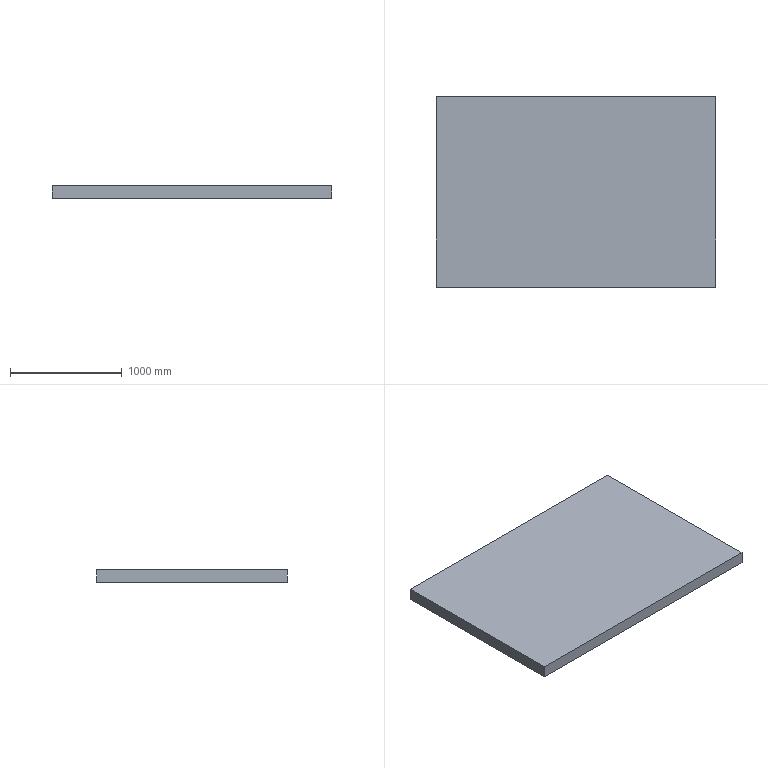Part | SolidWorks | features BaseBody 1 | 1 solid | 6 faces | box 2500 x 1700 x 110 mm | volume 467500000 mm3 | plane 6
STEP:
#1=CARTESIAN_POINT('',(1250.,-850.,0.));
#2=VERTEX_POINT('',#1);
#3=CARTESIAN_POINT('',(1250.,850.,0.));
#4=VERTEX_POINT('',#3);
#5=CARTESIAN_POINT('',(1250.,850.,0.));
#6=DIRECTION('',(0.,1.,0.));
#7=VECTOR('',#6,1000.);
#8=LINE('',#5,#7);
#9=EDGE_CURVE('',#2,#4,#8,.T.);
#10=ORIENTED_EDGE('',*,*,#9,.F.);
#11=CARTESIAN_POINT('',(-1250.,-850.,0.));
#12=VERTEX_POINT('',#11);
#13=CARTESIAN_POINT('',(-1250.,-850.,0.));
#14=DIRECTION('',(1.,0.,0.));
#15=VECTOR('',#14,1000.);
#16=LINE('',#13,#15);
#17=EDGE_CURVE('',#12,#2,#16,.T.);
#18=ORIENTED_EDGE('',*,*,#17,.F.);
#19=CARTESIAN_POINT('',(-1250.,850.,0.));
#20=VERTEX_POINT('',#19);
#21=CARTESIAN_POINT('',(-1250.,850.,0.));
#22=DIRECTION('',(0.,-1.,0.));
#23=VECTOR('',#22,1000.);
#24=LINE('',#21,#23);
#25=EDGE_CURVE('',#20,#12,#24,.T.);
#26=ORIENTED_EDGE('',*,*,#25,.F.);
#27=CARTESIAN_POINT('',(-1250.,850.,0.));
#28=DIRECTION('',(-1.,0.,0.));
#29=VECTOR('',#28,1000.);
#30=LINE('',#27,#29);
#31=EDGE_CURVE('',#4,#20,#30,.T.);
#32=ORIENTED_EDGE('',*,*,#31,.F.);
#33=EDGE_LOOP('',(#10,#18,#26,#32));
#34=FACE_OUTER_BOUND('',#33,.T.);
#35=CARTESIAN_POINT('',(0.,0.,0.));
#36=DIRECTION('',(0.,0.,1.));
#37=DIRECTION('',(1.,0.,0.));
#38=AXIS2_PLACEMENT_3D('',#35,#36,#37);
#39=PLANE('',#38);
#40=ADVANCED_FACE('',(#34),#39,.F.);
#41=CARTESIAN_POINT('',(1250.,-850.,110.));
#42=VERTEX_POINT('',#41);
#43=CARTESIAN_POINT('',(1250.,850.,110.));
#44=VERTEX_POINT('',#43);
#45=CARTESIAN_POINT('',(1250.,850.,110.));
#46=DIRECTION('',(0.,1.,0.));
#47=VECTOR('',#46,1000.);
#48=LINE('',#45,#47);
#49=EDGE_CURVE('',#42,#44,#48,.T.);
#50=ORIENTED_EDGE('',*,*,#49,.T.);
#51=CARTESIAN_POINT('',(-1250.,850.,110.));
#52=VERTEX_POINT('',#51);
#53=CARTESIAN_POINT('',(-1250.,850.,110.));
#54=DIRECTION('',(-1.,0.,0.));
#55=VECTOR('',#54,1000.);
#56=LINE('',#53,#55);
#57=EDGE_CURVE('',#44,#52,#56,.T.);
#58=ORIENTED_EDGE('',*,*,#57,.T.);
#59=CARTESIAN_POINT('',(-1250.,-850.,110.));
#60=VERTEX_POINT('',#59);
#61=CARTESIAN_POINT('',(-1250.,850.,110.));
#62=DIRECTION('',(0.,-1.,0.));
#63=VECTOR('',#62,1000.);
#64=LINE('',#61,#63);
#65=EDGE_CURVE('',#52,#60,#64,.T.);
#66=ORIENTED_EDGE('',*,*,#65,.T.);
#67=CARTESIAN_POINT('',(-1250.,-850.,110.));
#68=DIRECTION('',(1.,0.,0.));
#69=VECTOR('',#68,1000.);
#70=LINE('',#67,#69);
#71=EDGE_CURVE('',#60,#42,#70,.T.);
#72=ORIENTED_EDGE('',*,*,#71,.T.);
#73=EDGE_LOOP('',(#50,#58,#66,#72));
#74=FACE_OUTER_BOUND('',#73,.T.);
#75=CARTESIAN_POINT('',(0.,0.,110.));
#76=DIRECTION('',(0.,0.,1.));
#77=DIRECTION('',(1.,0.,0.));
#78=AXIS2_PLACEMENT_3D('',#75,#76,#77);
#79=PLANE('',#78);
#80=ADVANCED_FACE('',(#74),#79,.T.);
#81=ORIENTED_EDGE('',*,*,#17,.T.);
#82=CARTESIAN_POINT('',(1250.,-850.,110.));
#83=DIRECTION('',(0.,0.,-1.));
#84=VECTOR('',#83,1000.);
#85=LINE('',#82,#84);
#86=EDGE_CURVE('',#42,#2,#85,.T.);
#87=ORIENTED_EDGE('',*,*,#86,.F.);
#88=ORIENTED_EDGE('',*,*,#71,.F.);
#89=CARTESIAN_POINT('',(-1250.,-850.,110.));
#90=DIRECTION('',(0.,0.,-1.));
#91=VECTOR('',#90,1000.);
#92=LINE('',#89,#91);
#93=EDGE_CURVE('',#60,#12,#92,.T.);
#94=ORIENTED_EDGE('',*,*,#93,.T.);
#95=EDGE_LOOP('',(#81,#87,#88,#94));
#96=FACE_OUTER_BOUND('',#95,.T.);
#97=CARTESIAN_POINT('',(-1250.,-850.,110.));
#98=DIRECTION('',(0.,1.,0.));
#99=DIRECTION('',(1.,0.,0.));
#100=AXIS2_PLACEMENT_3D('',#97,#98,#99);
#101=PLANE('',#100);
#102=ADVANCED_FACE('',(#96),#101,.F.);
#103=ORIENTED_EDGE('',*,*,#25,.T.);
#104=ORIENTED_EDGE('',*,*,#93,.F.);
#105=ORIENTED_EDGE('',*,*,#65,.F.);
#106=CARTESIAN_POINT('',(-1250.,850.,110.));
#107=DIRECTION('',(0.,0.,-1.));
#108=VECTOR('',#107,1000.);
#109=LINE('',#106,#108);
#110=EDGE_CURVE('',#52,#20,#109,.T.);
#111=ORIENTED_EDGE('',*,*,#110,.T.);
#112=EDGE_LOOP('',(#103,#104,#105,#111));
#113=FACE_OUTER_BOUND('',#112,.T.);
#114=CARTESIAN_POINT('',(-1250.,850.,110.));
#115=DIRECTION('',(1.,0.,0.));
#116=DIRECTION('',(0.,1.,0.));
#117=AXIS2_PLACEMENT_3D('',#114,#115,#116);
#118=PLANE('',#117);
#119=ADVANCED_FACE('',(#113),#118,.F.);
#120=ORIENTED_EDGE('',*,*,#31,.T.);
#121=ORIENTED_EDGE('',*,*,#110,.F.);
#122=ORIENTED_EDGE('',*,*,#57,.F.);
#123=CARTESIAN_POINT('',(1250.,850.,110.));
#124=DIRECTION('',(0.,0.,-1.));
#125=VECTOR('',#124,1000.);
#126=LINE('',#123,#125);
#127=EDGE_CURVE('',#44,#4,#126,.T.);
#128=ORIENTED_EDGE('',*,*,#127,.T.);
#129=EDGE_LOOP('',(#120,#121,#122,#128));
#130=FACE_OUTER_BOUND('',#129,.T.);
#131=CARTESIAN_POINT('',(-1250.,850.,110.));
#132=DIRECTION('',(0.,-1.,0.));
#133=DIRECTION('',(0.,0.,-1.));
#134=AXIS2_PLACEMENT_3D('',#131,#132,#133);
#135=PLANE('',#134);
#136=ADVANCED_FACE('',(#130),#135,.F.);
#137=ORIENTED_EDGE('',*,*,#9,.T.);
#138=ORIENTED_EDGE('',*,*,#127,.F.);
#139=ORIENTED_EDGE('',*,*,#49,.F.);
#140=ORIENTED_EDGE('',*,*,#86,.T.);
#141=EDGE_LOOP('',(#137,#138,#139,#140));
#142=FACE_OUTER_BOUND('',#141,.T.);
#143=CARTESIAN_POINT('',(1250.,850.,110.));
#144=DIRECTION('',(-1.,0.,0.));
#145=DIRECTION('',(0.,0.,1.));
#146=AXIS2_PLACEMENT_3D('',#143,#144,#145);
#147=PLANE('',#146);
#148=ADVANCED_FACE('',(#142),#147,.F.);
#149=CLOSED_SHELL('',(#40,#80,#102,#119,#136,#148));
#150=MANIFOLD_SOLID_BREP('',#149);
#151=CARTESIAN_POINT('',(0.,0.,0.));
#152=DIRECTION('',(0.,0.,1.));
#153=DIRECTION('',(1.,0.,0.));
#154=AXIS2_PLACEMENT_3D('',#151,#152,#153);
#155=(LENGTH_UNIT()NAMED_UNIT(*)SI_UNIT(.MILLI.,.METRE.));
#156=UNCERTAINTY_MEASURE_WITH_UNIT(LENGTH_MEASURE(0.00001),#155,'','');
#157=(NAMED_UNIT(*)PLANE_ANGLE_UNIT()SI_UNIT($,.RADIAN.));
#158=(NAMED_UNIT(*)SI_UNIT($,.STERADIAN.)SOLID_ANGLE_UNIT());
#159=(GEOMETRIC_REPRESENTATION_CONTEXT(3)GLOBAL_UNCERTAINTY_ASSIGNED_CONTEXT((#156))GLOBAL_UNIT_ASSIGNED_CONTEXT((#155,#157,#158))REPRESENTATION_CONTEXT('',''));
#160=ADVANCED_BREP_SHAPE_REPRESENTATION('',(#150,#154),#159);